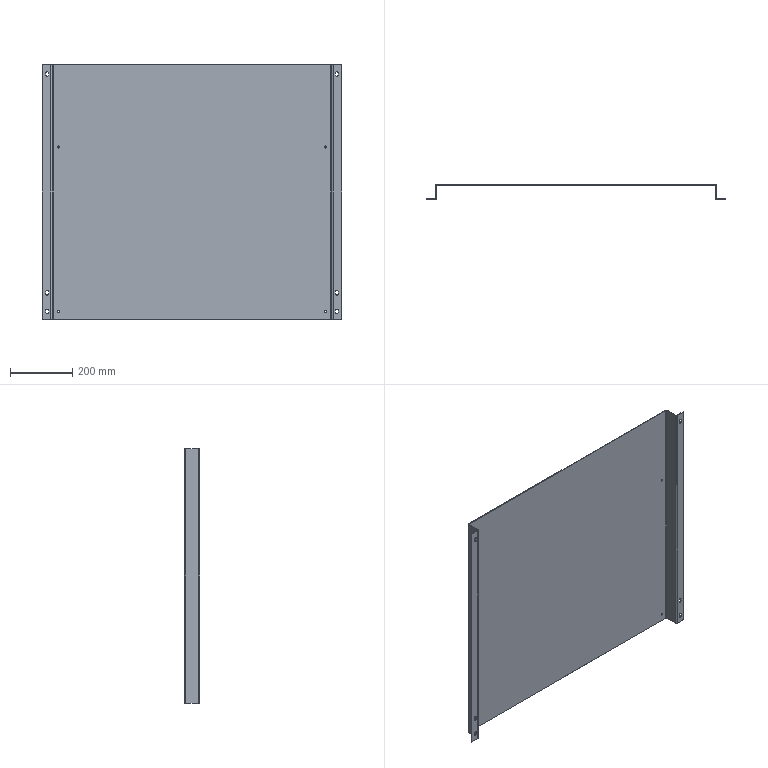Part | SolidWorks | features ICE 2, Extrusion 1 | 1 solid | 60 faces | box 966 x 49 x 820 mm | volume 2585319 mm3 | cylinder 34 | plane 26 | commonest cylinder face diameters 9 x18 7 x8 4 x4 10 x4